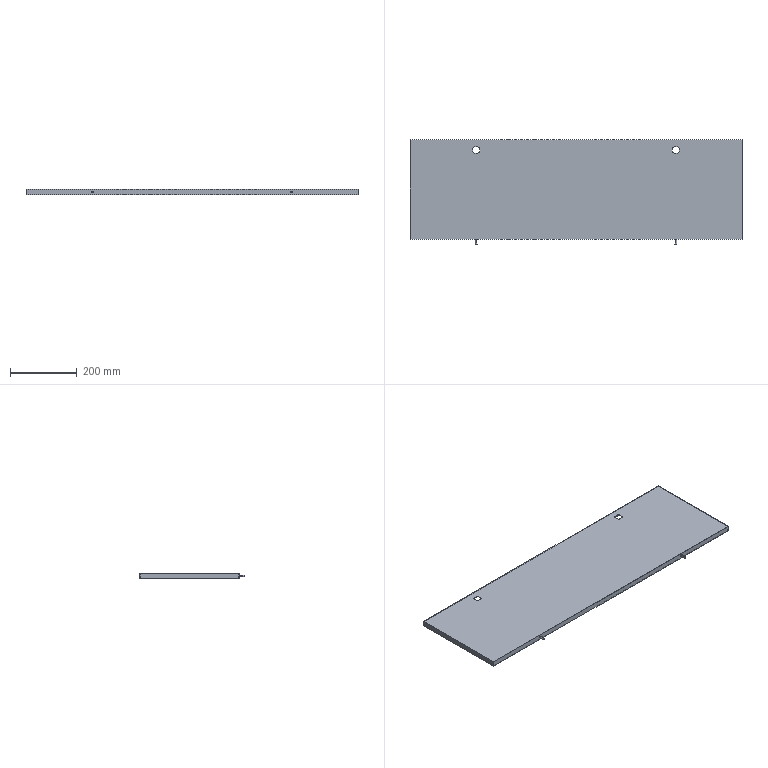Part | STEP file | 1 solid | 38 faces | box 998 x 313 x 16 mm | volume 527029 mm3 | plane 26 | cylinder 12 | commonest cylinder face diameters 22 x8 6 x4